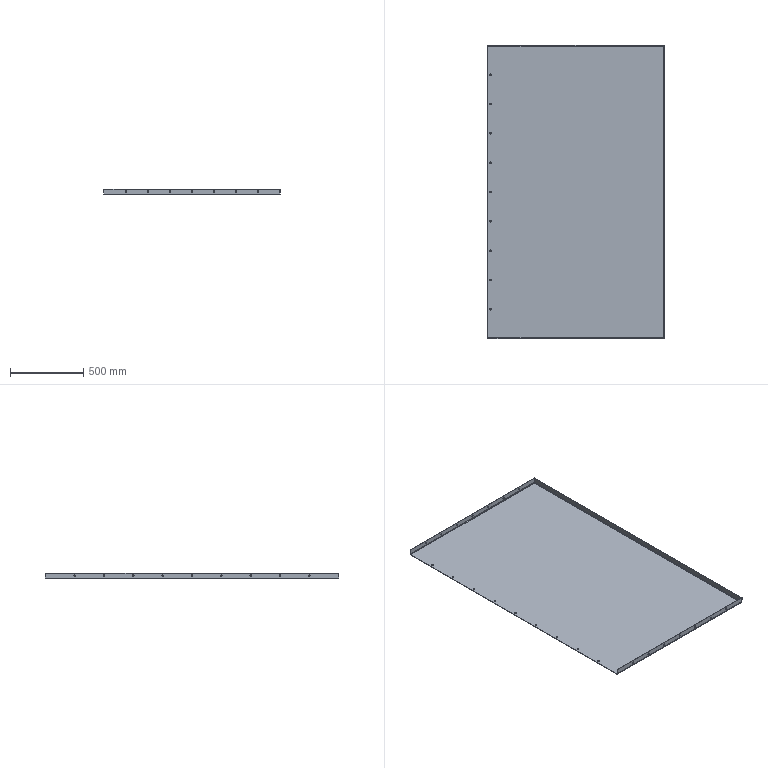Part | SolidWorks | features ICE 3, CornerFeat 1, EdgeFlange 1, FlatPattern 1, SMBaseFlange 1, SheetMetal 1 | 1 solid | 94 faces | box 1200 x 2000 x 40 mm | volume 7654629 mm3 | cylinder 70 | plane 20 | spline 4 | commonest cylinder face diameters 10 x64 6 x3 12 x3